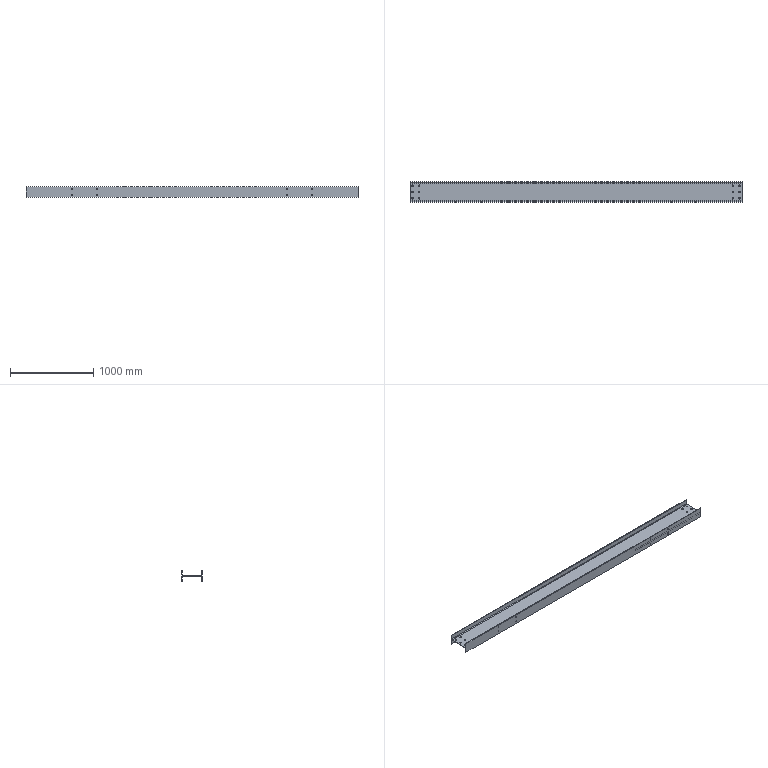Part | STEP file | 计量主梁1主体_Default<As Machined> | 1 solid | 58 faces | box 3986 x 250 x 125 mm | volume 14702858 mm3 | cylinder 44 | plane 14 | commonest cylinder face diameters 19 x24 15 x16 16 x4